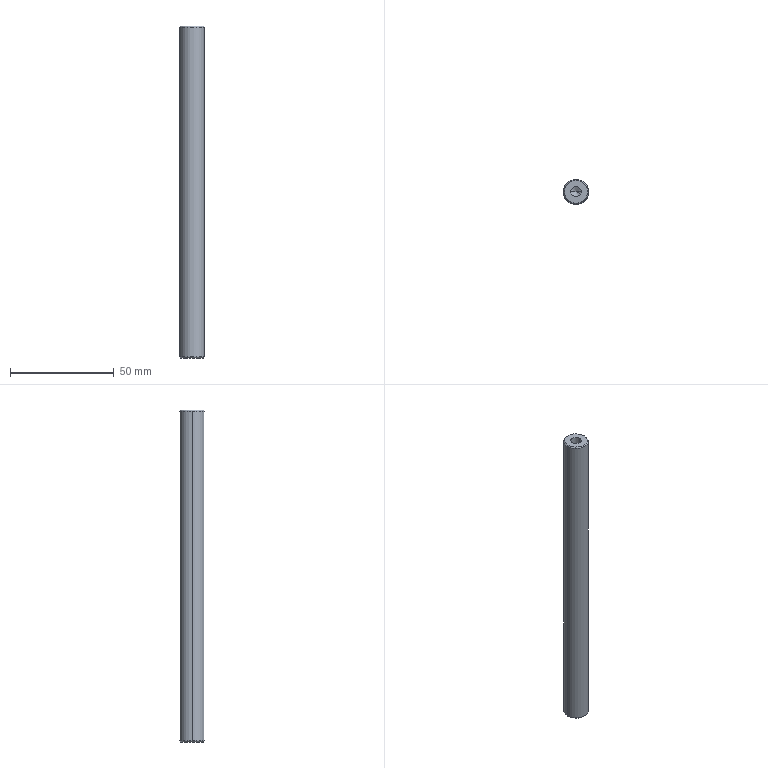Part | SolidWorks | features Chamfer 1, Extrusion 1, HoleWzd 1 | 1 solid | 12 faces | box 12 x 12 x 160 mm | volume 17782 mm3 | cone 6 | cylinder 4 | plane 2 | commonest cylinder face diameters 5 x2 12 x2
STEP:
#1=CARTESIAN_POINT('',(5.5,0.,160.));
#2=VERTEX_POINT('',#1);
#3=CARTESIAN_POINT('',(-5.5,0.,160.));
#4=VERTEX_POINT('',#3);
#5=CARTESIAN_POINT('',(0.,0.,160.));
#6=DIRECTION('',(0.,0.,1.));
#7=DIRECTION('',(1.,0.,0.));
#8=AXIS2_PLACEMENT_3D('',#5,#6,#7);
#9=CIRCLE('',#8,5.5);
#10=EDGE_CURVE('',#2,#4,#9,.T.);
#11=ORIENTED_EDGE('',*,*,#10,.F.);
#12=CARTESIAN_POINT('',(6.,0.,159.5));
#13=VERTEX_POINT('',#12);
#14=CARTESIAN_POINT('',(5.5,0.,160.));
#15=DIRECTION('',(0.7071,0.,-0.7071));
#16=VECTOR('',#15,1000.);
#17=LINE('',#14,#16);
#18=EDGE_CURVE('',#2,#13,#17,.T.);
#19=ORIENTED_EDGE('',*,*,#18,.T.);
#20=CARTESIAN_POINT('',(-6.,0.,159.5));
#21=VERTEX_POINT('',#20);
#22=CARTESIAN_POINT('',(0.,0.,159.5));
#23=DIRECTION('',(0.,0.,-1.));
#24=DIRECTION('',(1.,0.,0.));
#25=AXIS2_PLACEMENT_3D('',#22,#23,#24);
#26=CIRCLE('',#25,6.);
#27=EDGE_CURVE('',#21,#13,#26,.T.);
#28=ORIENTED_EDGE('',*,*,#27,.F.);
#29=CARTESIAN_POINT('',(-5.5,0.,160.));
#30=DIRECTION('',(-0.7071,0.,-0.7071));
#31=VECTOR('',#30,1000.);
#32=LINE('',#29,#31);
#33=EDGE_CURVE('',#4,#21,#32,.T.);
#34=ORIENTED_EDGE('',*,*,#33,.F.);
#35=EDGE_LOOP('',(#11,#19,#28,#34));
#36=FACE_OUTER_BOUND('',#35,.T.);
#37=CARTESIAN_POINT('',(0.,0.,160.));
#38=DIRECTION('',(0.,0.,-1.));
#39=DIRECTION('',(-1.,0.,0.));
#40=AXIS2_PLACEMENT_3D('',#37,#38,#39);
#41=CONICAL_SURFACE('',#40,5.5,0.7854);
#42=ADVANCED_FACE('',(#36),#41,.T.);
#43=CARTESIAN_POINT('',(-5.5,0.,0.));
#44=VERTEX_POINT('',#43);
#45=CARTESIAN_POINT('',(5.5,0.,0.));
#46=VERTEX_POINT('',#45);
#47=CARTESIAN_POINT('',(0.,0.,0.));
#48=DIRECTION('',(0.,0.,-1.));
#49=DIRECTION('',(1.,0.,0.));
#50=AXIS2_PLACEMENT_3D('',#47,#48,#49);
#51=CIRCLE('',#50,5.5);
#52=EDGE_CURVE('',#44,#46,#51,.T.);
#53=ORIENTED_EDGE('',*,*,#52,.F.);
#54=CARTESIAN_POINT('',(-6.,0.,0.5));
#55=VERTEX_POINT('',#54);
#56=CARTESIAN_POINT('',(-6.,0.,0.5));
#57=DIRECTION('',(-0.7071,0.,0.7071));
#58=VECTOR('',#57,1000.);
#59=LINE('',#56,#58);
#60=EDGE_CURVE('',#44,#55,#59,.T.);
#61=ORIENTED_EDGE('',*,*,#60,.T.);
#62=CARTESIAN_POINT('',(6.,0.,0.5));
#63=VERTEX_POINT('',#62);
#64=CARTESIAN_POINT('',(0.,0.,0.5));
#65=DIRECTION('',(0.,0.,1.));
#66=DIRECTION('',(1.,0.,0.));
#67=AXIS2_PLACEMENT_3D('',#64,#65,#66);
#68=CIRCLE('',#67,6.);
#69=EDGE_CURVE('',#63,#55,#68,.T.);
#70=ORIENTED_EDGE('',*,*,#69,.F.);
#71=CARTESIAN_POINT('',(6.,0.,0.5));
#72=DIRECTION('',(0.7071,0.,0.7071));
#73=VECTOR('',#72,1000.);
#74=LINE('',#71,#73);
#75=EDGE_CURVE('',#46,#63,#74,.T.);
#76=ORIENTED_EDGE('',*,*,#75,.F.);
#77=EDGE_LOOP('',(#53,#61,#70,#76));
#78=FACE_OUTER_BOUND('',#77,.T.);
#79=CARTESIAN_POINT('',(0.,0.,0.5));
#80=DIRECTION('',(0.,0.,1.));
#81=DIRECTION('',(1.,0.,0.));
#82=AXIS2_PLACEMENT_3D('',#79,#80,#81);
#83=CONICAL_SURFACE('',#82,6.,0.7854);
#84=ADVANCED_FACE('',(#78),#83,.T.);
#85=CARTESIAN_POINT('',(-2.5,0.,145.));
#86=VERTEX_POINT('',#85);
#87=CARTESIAN_POINT('',(2.5,0.,145.));
#88=VERTEX_POINT('',#87);
#89=CARTESIAN_POINT('',(0.,0.,145.));
#90=DIRECTION('',(0.,0.,1.));
#91=DIRECTION('',(1.,0.,0.));
#92=AXIS2_PLACEMENT_3D('',#89,#90,#91);
#93=CIRCLE('',#92,2.5);
#94=EDGE_CURVE('',#86,#88,#93,.T.);
#95=ORIENTED_EDGE('',*,*,#94,.F.);
#96=CARTESIAN_POINT('',(-2.5,0.,160.));
#97=VERTEX_POINT('',#96);
#98=CARTESIAN_POINT('',(-2.5,0.,160.));
#99=DIRECTION('',(0.,0.,1.));
#100=VECTOR('',#99,1000.);
#101=LINE('',#98,#100);
#102=EDGE_CURVE('',#86,#97,#101,.T.);
#103=ORIENTED_EDGE('',*,*,#102,.T.);
#104=CARTESIAN_POINT('',(2.5,0.,160.));
#105=VERTEX_POINT('',#104);
#106=CARTESIAN_POINT('',(0.,0.,160.));
#107=DIRECTION('',(0.,0.,1.));
#108=DIRECTION('',(1.,0.,0.));
#109=AXIS2_PLACEMENT_3D('',#106,#107,#108);
#110=CIRCLE('',#109,2.5);
#111=EDGE_CURVE('',#97,#105,#110,.T.);
#112=ORIENTED_EDGE('',*,*,#111,.T.);
#113=CARTESIAN_POINT('',(2.5,0.,160.));
#114=DIRECTION('',(0.,0.,1.));
#115=VECTOR('',#114,1000.);
#116=LINE('',#113,#115);
#117=EDGE_CURVE('',#88,#105,#116,.T.);
#118=ORIENTED_EDGE('',*,*,#117,.F.);
#119=EDGE_LOOP('',(#95,#103,#112,#118));
#120=FACE_OUTER_BOUND('',#119,.T.);
#121=CARTESIAN_POINT('',(0.,0.,160.));
#122=DIRECTION('',(0.,0.,1.));
#123=DIRECTION('',(1.,0.,0.));
#124=AXIS2_PLACEMENT_3D('',#121,#122,#123);
#125=CYLINDRICAL_SURFACE('',#124,2.5);
#126=ADVANCED_FACE('',(#120),#125,.F.);
#127=CARTESIAN_POINT('',(0.,0.,143.498));
#128=VERTEX_POINT('',#127);
#129=CARTESIAN_POINT('',(2.5,0.,145.));
#130=DIRECTION('',(0.8572,0.,0.515));
#131=VECTOR('',#130,1000.);
#132=LINE('',#129,#131);
#133=EDGE_CURVE('',#128,#88,#132,.T.);
#134=ORIENTED_EDGE('',*,*,#133,.F.);
#135=CARTESIAN_POINT('',(-2.5,0.,145.));
#136=DIRECTION('',(-0.8572,0.,0.515));
#137=VECTOR('',#136,1000.);
#138=LINE('',#135,#137);
#139=EDGE_CURVE('',#128,#86,#138,.T.);
#140=ORIENTED_EDGE('',*,*,#139,.T.);
#141=ORIENTED_EDGE('',*,*,#94,.T.);
#142=EDGE_LOOP('',(#134,#140,#141));
#143=FACE_OUTER_BOUND('',#142,.T.);
#144=CARTESIAN_POINT('',(0.,0.,145.));
#145=DIRECTION('',(0.,0.,1.));
#146=DIRECTION('',(1.,0.,0.));
#147=AXIS2_PLACEMENT_3D('',#144,#145,#146);
#148=CONICAL_SURFACE('',#147,2.5,1.03);
#149=ADVANCED_FACE('',(#143),#148,.F.);
#150=ORIENTED_EDGE('',*,*,#27,.T.);
#151=CARTESIAN_POINT('',(6.,0.,160.));
#152=DIRECTION('',(0.,0.,-1.));
#153=VECTOR('',#152,1000.);
#154=LINE('',#151,#153);
#155=EDGE_CURVE('',#13,#63,#154,.T.);
#156=ORIENTED_EDGE('',*,*,#155,.T.);
#157=ORIENTED_EDGE('',*,*,#69,.T.);
#158=CARTESIAN_POINT('',(-6.,0.,160.));
#159=DIRECTION('',(0.,0.,-1.));
#160=VECTOR('',#159,1000.);
#161=LINE('',#158,#160);
#162=EDGE_CURVE('',#21,#55,#161,.T.);
#163=ORIENTED_EDGE('',*,*,#162,.F.);
#164=EDGE_LOOP('',(#150,#156,#157,#163));
#165=FACE_OUTER_BOUND('',#164,.T.);
#166=CARTESIAN_POINT('',(0.,0.,160.));
#167=DIRECTION('',(0.,0.,-1.));
#168=DIRECTION('',(-1.,0.,0.));
#169=AXIS2_PLACEMENT_3D('',#166,#167,#168);
#170=CYLINDRICAL_SURFACE('',#169,6.);
#171=ADVANCED_FACE('',(#165),#170,.T.);
#172=ORIENTED_EDGE('',*,*,#155,.F.);
#173=CARTESIAN_POINT('',(0.,0.,159.5));
#174=DIRECTION('',(0.,0.,-1.));
#175=DIRECTION('',(1.,0.,0.));
#176=AXIS2_PLACEMENT_3D('',#173,#174,#175);
#177=CIRCLE('',#176,6.);
#178=EDGE_CURVE('',#13,#21,#177,.T.);
#179=ORIENTED_EDGE('',*,*,#178,.T.);
#180=ORIENTED_EDGE('',*,*,#162,.T.);
#181=CARTESIAN_POINT('',(0.,0.,0.5));
#182=DIRECTION('',(0.,0.,1.));
#183=DIRECTION('',(1.,0.,0.));
#184=AXIS2_PLACEMENT_3D('',#181,#182,#183);
#185=CIRCLE('',#184,6.);
#186=EDGE_CURVE('',#55,#63,#185,.T.);
#187=ORIENTED_EDGE('',*,*,#186,.T.);
#188=EDGE_LOOP('',(#172,#179,#180,#187));
#189=FACE_OUTER_BOUND('',#188,.T.);
#190=CARTESIAN_POINT('',(0.,0.,160.));
#191=DIRECTION('',(0.,0.,-1.));
#192=DIRECTION('',(-1.,0.,0.));
#193=AXIS2_PLACEMENT_3D('',#190,#191,#192);
#194=CYLINDRICAL_SURFACE('',#193,6.);
#195=ADVANCED_FACE('',(#189),#194,.T.);
#196=CARTESIAN_POINT('',(0.,0.,160.));
#197=DIRECTION('',(0.,0.,1.));
#198=DIRECTION('',(1.,0.,0.));
#199=AXIS2_PLACEMENT_3D('',#196,#197,#198);
#200=CIRCLE('',#199,5.5);
#201=EDGE_CURVE('',#4,#2,#200,.T.);
#202=ORIENTED_EDGE('',*,*,#201,.T.);
#203=ORIENTED_EDGE('',*,*,#10,.T.);
#204=EDGE_LOOP('',(#202,#203));
#205=FACE_OUTER_BOUND('',#204,.T.);
#206=CARTESIAN_POINT('',(0.,0.,160.));
#207=DIRECTION('',(0.,0.,1.));
#208=DIRECTION('',(1.,0.,0.));
#209=AXIS2_PLACEMENT_3D('',#206,#207,#208);
#210=CIRCLE('',#209,2.5);
#211=EDGE_CURVE('',#105,#97,#210,.T.);
#212=ORIENTED_EDGE('',*,*,#211,.F.);
#213=ORIENTED_EDGE('',*,*,#111,.F.);
#214=EDGE_LOOP('',(#212,#213));
#215=FACE_BOUND('',#214,.T.);
#216=CARTESIAN_POINT('',(0.,0.,160.));
#217=DIRECTION('',(0.,0.,1.));
#218=DIRECTION('',(1.,0.,0.));
#219=AXIS2_PLACEMENT_3D('',#216,#217,#218);
#220=PLANE('',#219);
#221=ADVANCED_FACE('',(#205,#215),#220,.T.);
#222=CARTESIAN_POINT('',(0.,0.,0.));
#223=DIRECTION('',(0.,0.,-1.));
#224=DIRECTION('',(1.,0.,0.));
#225=AXIS2_PLACEMENT_3D('',#222,#223,#224);
#226=CIRCLE('',#225,5.5);
#227=EDGE_CURVE('',#46,#44,#226,.T.);
#228=ORIENTED_EDGE('',*,*,#227,.T.);
#229=ORIENTED_EDGE('',*,*,#52,.T.);
#230=EDGE_LOOP('',(#228,#229));
#231=FACE_OUTER_BOUND('',#230,.T.);
#232=CARTESIAN_POINT('',(0.,0.,0.));
#233=DIRECTION('',(0.,0.,1.));
#234=DIRECTION('',(1.,0.,0.));
#235=AXIS2_PLACEMENT_3D('',#232,#233,#234);
#236=PLANE('',#235);
#237=ADVANCED_FACE('',(#231),#236,.F.);
#238=ORIENTED_EDGE('',*,*,#139,.F.);
#239=ORIENTED_EDGE('',*,*,#133,.T.);
#240=CARTESIAN_POINT('',(0.,0.,145.));
#241=DIRECTION('',(0.,0.,1.));
#242=DIRECTION('',(1.,0.,0.));
#243=AXIS2_PLACEMENT_3D('',#240,#241,#242);
#244=CIRCLE('',#243,2.5);
#245=EDGE_CURVE('',#88,#86,#244,.T.);
#246=ORIENTED_EDGE('',*,*,#245,.T.);
#247=EDGE_LOOP('',(#238,#239,#246));
#248=FACE_OUTER_BOUND('',#247,.T.);
#249=CARTESIAN_POINT('',(0.,0.,145.));
#250=DIRECTION('',(0.,0.,1.));
#251=DIRECTION('',(1.,0.,0.));
#252=AXIS2_PLACEMENT_3D('',#249,#250,#251);
#253=CONICAL_SURFACE('',#252,2.5,1.03);
#254=ADVANCED_FACE('',(#248),#253,.F.);
#255=ORIENTED_EDGE('',*,*,#102,.F.);
#256=ORIENTED_EDGE('',*,*,#245,.F.);
#257=ORIENTED_EDGE('',*,*,#117,.T.);
#258=ORIENTED_EDGE('',*,*,#211,.T.);
#259=EDGE_LOOP('',(#255,#256,#257,#258));
#260=FACE_OUTER_BOUND('',#259,.T.);
#261=CARTESIAN_POINT('',(0.,0.,160.));
#262=DIRECTION('',(0.,0.,1.));
#263=DIRECTION('',(1.,0.,0.));
#264=AXIS2_PLACEMENT_3D('',#261,#262,#263);
#265=CYLINDRICAL_SURFACE('',#264,2.5);
#266=ADVANCED_FACE('',(#260),#265,.F.);
#267=ORIENTED_EDGE('',*,*,#60,.F.);
#268=ORIENTED_EDGE('',*,*,#227,.F.);
#269=ORIENTED_EDGE('',*,*,#75,.T.);
#270=ORIENTED_EDGE('',*,*,#186,.F.);
#271=EDGE_LOOP('',(#267,#268,#269,#270));
#272=FACE_OUTER_BOUND('',#271,.T.);
#273=CARTESIAN_POINT('',(0.,0.,0.5));
#274=DIRECTION('',(0.,0.,1.));
#275=DIRECTION('',(1.,0.,0.));
#276=AXIS2_PLACEMENT_3D('',#273,#274,#275);
#277=CONICAL_SURFACE('',#276,6.,0.7854);
#278=ADVANCED_FACE('',(#272),#277,.T.);
#279=ORIENTED_EDGE('',*,*,#18,.F.);
#280=ORIENTED_EDGE('',*,*,#201,.F.);
#281=ORIENTED_EDGE('',*,*,#33,.T.);
#282=ORIENTED_EDGE('',*,*,#178,.F.);
#283=EDGE_LOOP('',(#279,#280,#281,#282));
#284=FACE_OUTER_BOUND('',#283,.T.);
#285=CARTESIAN_POINT('',(0.,0.,160.));
#286=DIRECTION('',(0.,0.,-1.));
#287=DIRECTION('',(-1.,0.,0.));
#288=AXIS2_PLACEMENT_3D('',#285,#286,#287);
#289=CONICAL_SURFACE('',#288,5.5,0.7854);
#290=ADVANCED_FACE('',(#284),#289,.T.);
#291=CLOSED_SHELL('',(#42,#84,#126,#149,#171,#195,#221,#237,#254,#266,#278,#290));
#292=MANIFOLD_SOLID_BREP('',#291);
#293=CARTESIAN_POINT('',(0.,0.,0.));
#294=DIRECTION('',(0.,0.,1.));
#295=DIRECTION('',(1.,0.,0.));
#296=AXIS2_PLACEMENT_3D('',#293,#294,#295);
#297=(LENGTH_UNIT()NAMED_UNIT(*)SI_UNIT(.MILLI.,.METRE.));
#298=UNCERTAINTY_MEASURE_WITH_UNIT(LENGTH_MEASURE(0.00001),#297,'','');
#299=(NAMED_UNIT(*)PLANE_ANGLE_UNIT()SI_UNIT($,.RADIAN.));
#300=(NAMED_UNIT(*)SI_UNIT($,.STERADIAN.)SOLID_ANGLE_UNIT());
#301=(GEOMETRIC_REPRESENTATION_CONTEXT(3)GLOBAL_UNCERTAINTY_ASSIGNED_CONTEXT((#298))GLOBAL_UNIT_ASSIGNED_CONTEXT((#297,#299,#300))REPRESENTATION_CONTEXT('',''));
#302=ADVANCED_BREP_SHAPE_REPRESENTATION('',(#292,#296),#301);